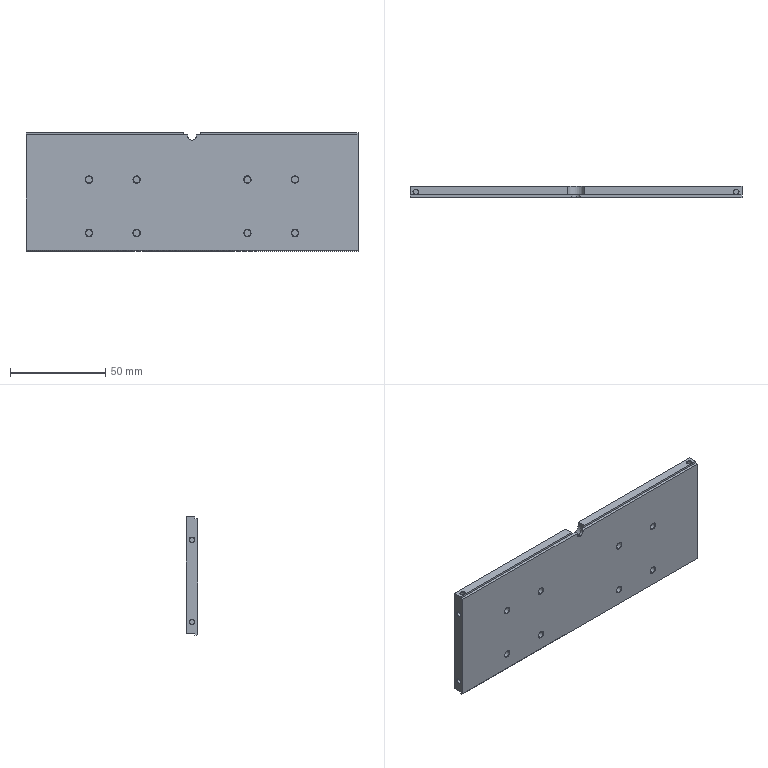Part | SolidWorks | features BaseBody 1 | 1 solid | 112 faces | box 174 x 6 x 62 mm | volume 62898 mm3 | cylinder 39 | plane 37 | cone 36 | commonest cylinder face diameters 3.5 x16 2.5 x12 1.6 x8 4.4 x2 9 x1